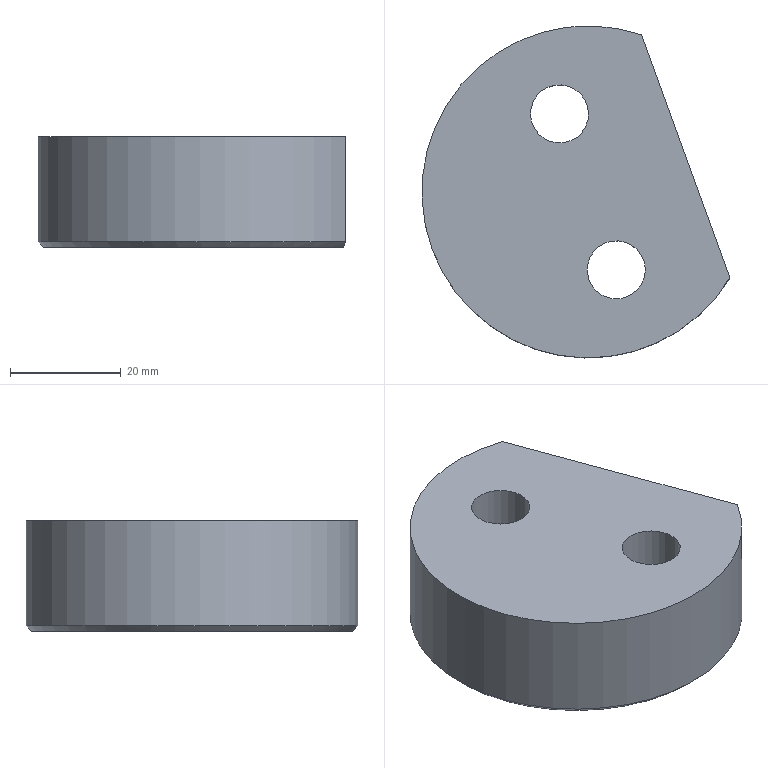Part | NX | features XD1540-60-20 2 | 1 solid | 13 faces | box 55.658 x 60 x 20 mm | volume 41796 mm3 | plane 5 | cylinder 5 | torus 2 | cone 1 | commonest cylinder face diameters 10.5 x2 17.5 x2 60 x1
STEP:
#1=CARTESIAN_POINT('',(385.107,-197.818,-380.));
#2=VERTEX_POINT('',#1);
#3=CARTESIAN_POINT('',(400.214,-239.326,-380.));
#4=VERTEX_POINT('',#3);
#5=CARTESIAN_POINT('',(392.66,-218.572,-380.));
#6=DIRECTION('',(0.342,-0.9397,0.));
#7=VECTOR('',#6,1000.);
#8=LINE('',#5,#7);
#9=EDGE_CURVE('',#2,#4,#8,.T.);
#10=ORIENTED_EDGE('',*,*,#9,.T.);
#11=CARTESIAN_POINT('',(375.,-225.,-380.));
#12=DIRECTION('',(0.,0.,1.));
#13=DIRECTION('',(0.9063,-0.4226,0.));
#14=AXIS2_PLACEMENT_3D('',#11,#12,#13);
#15=CIRCLE('',#14,29.);
#16=EDGE_CURVE('',#2,#4,#15,.T.);
#17=ORIENTED_EDGE('',*,*,#16,.F.);
#18=EDGE_LOOP('',(#10,#17));
#19=FACE_BOUND('',#18,.T.);
#20=CARTESIAN_POINT('',(390.779,-244.061,-380.));
#21=VERTEX_POINT('',#20);
#22=CARTESIAN_POINT('',(380.13,-239.095,-380.));
#23=DIRECTION('',(0.,0.,-1.));
#24=DIRECTION('',(0.9063,-0.4226,0.));
#25=AXIS2_PLACEMENT_3D('',#22,#23,#24);
#26=CIRCLE('',#25,11.75);
#27=EDGE_CURVE('',#21,#21,#26,.T.);
#28=ORIENTED_EDGE('',*,*,#27,.F.);
#29=EDGE_LOOP('',(#28));
#30=FACE_BOUND('',#29,.T.);
#31=CARTESIAN_POINT('',(380.519,-215.87,-380.));
#32=VERTEX_POINT('',#31);
#33=CARTESIAN_POINT('',(369.87,-210.905,-380.));
#34=DIRECTION('',(0.,0.,-1.));
#35=DIRECTION('',(0.9063,-0.4226,0.));
#36=AXIS2_PLACEMENT_3D('',#33,#34,#35);
#37=CIRCLE('',#36,11.75);
#38=EDGE_CURVE('',#32,#32,#37,.T.);
#39=ORIENTED_EDGE('',*,*,#38,.F.);
#40=EDGE_LOOP('',(#39));
#41=FACE_BOUND('',#40,.T.);
#42=CARTESIAN_POINT('',(375.,-225.,-380.));
#43=DIRECTION('',(0.,0.,-1.));
#44=DIRECTION('',(-0.9063,0.4226,0.));
#45=AXIS2_PLACEMENT_3D('',#42,#43,#44);
#46=PLANE('',#45);
#47=ADVANCED_FACE('',(#19,#30,#41),#46,.T.);
#48=CARTESIAN_POINT('',(400.658,-240.545,-360.));
#49=VERTEX_POINT('',#48);
#50=CARTESIAN_POINT('',(384.663,-196.599,-360.));
#51=VERTEX_POINT('',#50);
#52=CARTESIAN_POINT('',(392.66,-218.572,-360.));
#53=DIRECTION('',(-0.342,0.9397,0.));
#54=VECTOR('',#53,1000.);
#55=LINE('',#52,#54);
#56=EDGE_CURVE('',#49,#51,#55,.T.);
#57=ORIENTED_EDGE('',*,*,#56,.T.);
#58=CARTESIAN_POINT('',(375.,-225.,-360.));
#59=DIRECTION('',(0.,0.,1.));
#60=DIRECTION('',(0.9063,-0.4226,0.));
#61=AXIS2_PLACEMENT_3D('',#58,#59,#60);
#62=CIRCLE('',#61,30.);
#63=EDGE_CURVE('',#51,#49,#62,.T.);
#64=ORIENTED_EDGE('',*,*,#63,.T.);
#65=EDGE_LOOP('',(#57,#64));
#66=FACE_BOUND('',#65,.T.);
#67=CARTESIAN_POINT('',(375.372,-236.877,-360.));
#68=VERTEX_POINT('',#67);
#69=CARTESIAN_POINT('',(380.13,-239.095,-360.));
#70=DIRECTION('',(0.,0.,-1.));
#71=DIRECTION('',(-0.9063,0.4226,0.));
#72=AXIS2_PLACEMENT_3D('',#69,#70,#71);
#73=CIRCLE('',#72,5.25);
#74=EDGE_CURVE('',#68,#68,#73,.T.);
#75=ORIENTED_EDGE('',*,*,#74,.T.);
#76=EDGE_LOOP('',(#75));
#77=FACE_BOUND('',#76,.T.);
#78=CARTESIAN_POINT('',(365.112,-208.686,-360.));
#79=VERTEX_POINT('',#78);
#80=CARTESIAN_POINT('',(369.87,-210.905,-360.));
#81=DIRECTION('',(0.,0.,-1.));
#82=DIRECTION('',(-0.9063,0.4226,0.));
#83=AXIS2_PLACEMENT_3D('',#80,#81,#82);
#84=CIRCLE('',#83,5.25);
#85=EDGE_CURVE('',#79,#79,#84,.T.);
#86=ORIENTED_EDGE('',*,*,#85,.T.);
#87=EDGE_LOOP('',(#86));
#88=FACE_BOUND('',#87,.T.);
#89=CARTESIAN_POINT('',(375.,-225.,-360.));
#90=DIRECTION('',(0.,0.,1.));
#91=DIRECTION('',(0.9063,-0.4226,0.));
#92=AXIS2_PLACEMENT_3D('',#89,#90,#91);
#93=PLANE('',#92);
#94=ADVANCED_FACE('',(#66,#77,#88),#93,.T.);
#95=CARTESIAN_POINT('',(400.658,-240.545,-379.));
#96=VERTEX_POINT('',#95);
#97=CARTESIAN_POINT('',(400.658,-240.545,-360.));
#98=DIRECTION('',(0.,0.,1.));
#99=VECTOR('',#98,1000.);
#100=LINE('',#97,#99);
#101=EDGE_CURVE('',#96,#49,#100,.T.);
#102=ORIENTED_EDGE('',*,*,#101,.T.);
#103=ORIENTED_EDGE('',*,*,#63,.F.);
#104=CARTESIAN_POINT('',(384.663,-196.599,-379.));
#105=VERTEX_POINT('',#104);
#106=CARTESIAN_POINT('',(384.663,-196.599,-360.));
#107=DIRECTION('',(0.,0.,-1.));
#108=VECTOR('',#107,1000.);
#109=LINE('',#106,#108);
#110=EDGE_CURVE('',#51,#105,#109,.T.);
#111=ORIENTED_EDGE('',*,*,#110,.T.);
#112=CARTESIAN_POINT('',(375.,-225.,-379.));
#113=DIRECTION('',(0.,0.,-1.));
#114=DIRECTION('',(0.9063,-0.4226,0.));
#115=AXIS2_PLACEMENT_3D('',#112,#113,#114);
#116=CIRCLE('',#115,30.);
#117=EDGE_CURVE('',#96,#105,#116,.T.);
#118=ORIENTED_EDGE('',*,*,#117,.F.);
#119=EDGE_LOOP('',(#102,#103,#111,#118));
#120=FACE_BOUND('',#119,.T.);
#121=CARTESIAN_POINT('',(375.,-225.,-360.));
#122=DIRECTION('',(0.,0.,-1.));
#123=DIRECTION('',(-0.9063,0.4226,0.));
#124=AXIS2_PLACEMENT_3D('',#121,#122,#123);
#125=CYLINDRICAL_SURFACE('',#124,30.);
#126=ADVANCED_FACE('',(#120),#125,.T.);
#127=CARTESIAN_POINT('',(365.112,-208.686,-368.));
#128=VERTEX_POINT('',#127);
#129=CARTESIAN_POINT('',(369.87,-210.905,-368.));
#130=DIRECTION('',(0.,0.,-1.));
#131=DIRECTION('',(-0.9063,0.4226,0.));
#132=AXIS2_PLACEMENT_3D('',#129,#130,#131);
#133=CIRCLE('',#132,5.25);
#134=EDGE_CURVE('',#128,#128,#133,.T.);
#135=ORIENTED_EDGE('',*,*,#134,.F.);
#136=EDGE_LOOP('',(#135));
#137=FACE_BOUND('',#136,.T.);
#138=CARTESIAN_POINT('',(377.8,-214.603,-368.));
#139=VERTEX_POINT('',#138);
#140=CARTESIAN_POINT('',(369.87,-210.905,-368.));
#141=DIRECTION('',(0.,0.,1.));
#142=DIRECTION('',(0.9063,-0.4226,0.));
#143=AXIS2_PLACEMENT_3D('',#140,#141,#142);
#144=CIRCLE('',#143,8.75);
#145=EDGE_CURVE('',#139,#139,#144,.T.);
#146=ORIENTED_EDGE('',*,*,#145,.F.);
#147=EDGE_LOOP('',(#146));
#148=FACE_BOUND('',#147,.T.);
#149=CARTESIAN_POINT('',(369.87,-210.905,-368.));
#150=DIRECTION('',(0.,0.,1.));
#151=DIRECTION('',(0.9063,-0.4226,0.));
#152=AXIS2_PLACEMENT_3D('',#149,#150,#151);
#153=PLANE('',#152);
#154=ADVANCED_FACE('',(#137,#148),#153,.F.);
#155=CARTESIAN_POINT('',(377.8,-214.603,-377.));
#156=VERTEX_POINT('',#155);
#157=CARTESIAN_POINT('',(369.87,-210.905,-377.));
#158=DIRECTION('',(0.,0.,1.));
#159=DIRECTION('',(0.9063,-0.4226,0.));
#160=AXIS2_PLACEMENT_3D('',#157,#158,#159);
#161=CIRCLE('',#160,8.75);
#162=EDGE_CURVE('',#156,#156,#161,.T.);
#163=ORIENTED_EDGE('',*,*,#162,.F.);
#164=EDGE_LOOP('',(#163));
#165=FACE_BOUND('',#164,.T.);
#166=ORIENTED_EDGE('',*,*,#145,.T.);
#167=EDGE_LOOP('',(#166));
#168=FACE_BOUND('',#167,.T.);
#169=CARTESIAN_POINT('',(369.87,-210.905,-368.));
#170=DIRECTION('',(0.,0.,-1.));
#171=DIRECTION('',(-0.9063,0.4226,0.));
#172=AXIS2_PLACEMENT_3D('',#169,#170,#171);
#173=CYLINDRICAL_SURFACE('',#172,8.75);
#174=ADVANCED_FACE('',(#165,#168),#173,.F.);
#175=CARTESIAN_POINT('',(375.372,-236.877,-368.));
#176=VERTEX_POINT('',#175);
#177=CARTESIAN_POINT('',(380.13,-239.095,-368.));
#178=DIRECTION('',(0.,0.,-1.));
#179=DIRECTION('',(-0.9063,0.4226,0.));
#180=AXIS2_PLACEMENT_3D('',#177,#178,#179);
#181=CIRCLE('',#180,5.25);
#182=EDGE_CURVE('',#176,#176,#181,.T.);
#183=ORIENTED_EDGE('',*,*,#182,.F.);
#184=EDGE_LOOP('',(#183));
#185=FACE_BOUND('',#184,.T.);
#186=CARTESIAN_POINT('',(388.06,-242.793,-368.));
#187=VERTEX_POINT('',#186);
#188=CARTESIAN_POINT('',(380.13,-239.095,-368.));
#189=DIRECTION('',(0.,0.,1.));
#190=DIRECTION('',(0.9063,-0.4226,0.));
#191=AXIS2_PLACEMENT_3D('',#188,#189,#190);
#192=CIRCLE('',#191,8.75);
#193=EDGE_CURVE('',#187,#187,#192,.T.);
#194=ORIENTED_EDGE('',*,*,#193,.F.);
#195=EDGE_LOOP('',(#194));
#196=FACE_BOUND('',#195,.T.);
#197=CARTESIAN_POINT('',(380.13,-239.095,-368.));
#198=DIRECTION('',(0.,0.,1.));
#199=DIRECTION('',(0.9063,-0.4226,0.));
#200=AXIS2_PLACEMENT_3D('',#197,#198,#199);
#201=PLANE('',#200);
#202=ADVANCED_FACE('',(#185,#196),#201,.F.);
#203=CARTESIAN_POINT('',(388.06,-242.793,-377.));
#204=VERTEX_POINT('',#203);
#205=CARTESIAN_POINT('',(380.13,-239.095,-377.));
#206=DIRECTION('',(0.,0.,1.));
#207=DIRECTION('',(0.9063,-0.4226,0.));
#208=AXIS2_PLACEMENT_3D('',#205,#206,#207);
#209=CIRCLE('',#208,8.75);
#210=EDGE_CURVE('',#204,#204,#209,.T.);
#211=ORIENTED_EDGE('',*,*,#210,.F.);
#212=EDGE_LOOP('',(#211));
#213=FACE_BOUND('',#212,.T.);
#214=ORIENTED_EDGE('',*,*,#193,.T.);
#215=EDGE_LOOP('',(#214));
#216=FACE_BOUND('',#215,.T.);
#217=CARTESIAN_POINT('',(380.13,-239.095,-368.));
#218=DIRECTION('',(0.,0.,-1.));
#219=DIRECTION('',(-0.9063,0.4226,0.));
#220=AXIS2_PLACEMENT_3D('',#217,#218,#219);
#221=CYLINDRICAL_SURFACE('',#220,8.75);
#222=ADVANCED_FACE('',(#213,#216),#221,.F.);
#223=ORIENTED_EDGE('',*,*,#85,.F.);
#224=EDGE_LOOP('',(#223));
#225=FACE_BOUND('',#224,.T.);
#226=ORIENTED_EDGE('',*,*,#134,.T.);
#227=EDGE_LOOP('',(#226));
#228=FACE_BOUND('',#227,.T.);
#229=CARTESIAN_POINT('',(369.87,-210.905,-359.));
#230=DIRECTION('',(0.,0.,-1.));
#231=DIRECTION('',(-0.9063,0.4226,0.));
#232=AXIS2_PLACEMENT_3D('',#229,#230,#231);
#233=CYLINDRICAL_SURFACE('',#232,5.25);
#234=ADVANCED_FACE('',(#225,#228),#233,.F.);
#235=ORIENTED_EDGE('',*,*,#74,.F.);
#236=EDGE_LOOP('',(#235));
#237=FACE_BOUND('',#236,.T.);
#238=ORIENTED_EDGE('',*,*,#182,.T.);
#239=EDGE_LOOP('',(#238));
#240=FACE_BOUND('',#239,.T.);
#241=CARTESIAN_POINT('',(380.13,-239.095,-359.));
#242=DIRECTION('',(0.,0.,-1.));
#243=DIRECTION('',(-0.9063,0.4226,0.));
#244=AXIS2_PLACEMENT_3D('',#241,#242,#243);
#245=CYLINDRICAL_SURFACE('',#244,5.25);
#246=ADVANCED_FACE('',(#237,#240),#245,.F.);
#247=ORIENTED_EDGE('',*,*,#38,.T.);
#248=EDGE_LOOP('',(#247));
#249=FACE_BOUND('',#248,.T.);
#250=ORIENTED_EDGE('',*,*,#162,.T.);
#251=EDGE_LOOP('',(#250));
#252=FACE_BOUND('',#251,.T.);
#253=CARTESIAN_POINT('',(369.87,-210.905,-377.));
#254=DIRECTION('',(0.,0.,-1.));
#255=DIRECTION('',(-0.9063,0.4226,0.));
#256=AXIS2_PLACEMENT_3D('',#253,#254,#255);
#257=TOROIDAL_SURFACE('',#256,11.75,3.);
#258=ADVANCED_FACE('',(#249,#252),#257,.T.);
#259=ORIENTED_EDGE('',*,*,#27,.T.);
#260=EDGE_LOOP('',(#259));
#261=FACE_BOUND('',#260,.T.);
#262=ORIENTED_EDGE('',*,*,#210,.T.);
#263=EDGE_LOOP('',(#262));
#264=FACE_BOUND('',#263,.T.);
#265=CARTESIAN_POINT('',(380.13,-239.095,-377.));
#266=DIRECTION('',(0.,0.,-1.));
#267=DIRECTION('',(-0.9063,0.4226,0.));
#268=AXIS2_PLACEMENT_3D('',#265,#266,#267);
#269=TOROIDAL_SURFACE('',#268,11.75,3.);
#270=ADVANCED_FACE('',(#261,#264),#269,.T.);
#271=CARTESIAN_POINT('',(384.663,-196.599,-379.));
#272=CARTESIAN_POINT('',(384.81,-197.003,-379.336));
#273=CARTESIAN_POINT('',(384.958,-197.41,-379.669));
#274=CARTESIAN_POINT('',(385.107,-197.818,-380.));
#275=B_SPLINE_CURVE_WITH_KNOTS('',3,(#271,#272,#273,#274),.UNSPECIFIED.,.F.,.F.,(4,4),(0.,1.),.PIECEWISE_BEZIER_KNOTS.);
#276=EDGE_CURVE('',#105,#2,#275,.T.);
#277=ORIENTED_EDGE('',*,*,#276,.T.);
#278=ORIENTED_EDGE('',*,*,#16,.T.);
#279=CARTESIAN_POINT('',(400.214,-239.326,-380.));
#280=CARTESIAN_POINT('',(400.363,-239.734,-379.669));
#281=CARTESIAN_POINT('',(400.511,-240.141,-379.336));
#282=CARTESIAN_POINT('',(400.658,-240.545,-379.));
#283=B_SPLINE_CURVE_WITH_KNOTS('',3,(#279,#280,#281,#282),.UNSPECIFIED.,.F.,.F.,(4,4),(0.,1.),.PIECEWISE_BEZIER_KNOTS.);
#284=EDGE_CURVE('',#4,#96,#283,.T.);
#285=ORIENTED_EDGE('',*,*,#284,.T.);
#286=ORIENTED_EDGE('',*,*,#117,.T.);
#287=EDGE_LOOP('',(#277,#278,#285,#286));
#288=FACE_BOUND('',#287,.T.);
#289=CARTESIAN_POINT('',(375.,-225.,-379.));
#290=DIRECTION('',(0.,0.,1.));
#291=DIRECTION('',(0.9063,-0.4226,0.));
#292=AXIS2_PLACEMENT_3D('',#289,#290,#291);
#293=CONICAL_SURFACE('',#292,30.,0.7854);
#294=ADVANCED_FACE('',(#288),#293,.T.);
#295=ORIENTED_EDGE('',*,*,#110,.F.);
#296=ORIENTED_EDGE('',*,*,#56,.F.);
#297=ORIENTED_EDGE('',*,*,#101,.F.);
#298=ORIENTED_EDGE('',*,*,#284,.F.);
#299=ORIENTED_EDGE('',*,*,#9,.F.);
#300=ORIENTED_EDGE('',*,*,#276,.F.);
#301=EDGE_LOOP('',(#295,#296,#297,#298,#299,#300));
#302=FACE_BOUND('',#301,.T.);
#303=CARTESIAN_POINT('',(404.919,-252.251,-580.));
#304=DIRECTION('',(-0.9397,-0.342,0.));
#305=DIRECTION('',(0.342,-0.9397,0.));
#306=AXIS2_PLACEMENT_3D('',#303,#304,#305);
#307=PLANE('',#306);
#308=ADVANCED_FACE('',(#302),#307,.F.);
#309=CLOSED_SHELL('',(#47,#94,#126,#154,#174,#202,#222,#234,#246,#258,#270,#294,#308));
#310=MANIFOLD_SOLID_BREP('',#309);
#311=(LENGTH_UNIT()NAMED_UNIT(*)SI_UNIT(.MILLI.,.METRE.));
#312=UNCERTAINTY_MEASURE_WITH_UNIT(LENGTH_MEASURE(0.00001),#311,'','');
#313=(NAMED_UNIT(*)PLANE_ANGLE_UNIT()SI_UNIT($,.RADIAN.));
#314=(NAMED_UNIT(*)SI_UNIT($,.STERADIAN.)SOLID_ANGLE_UNIT());
#315=(GEOMETRIC_REPRESENTATION_CONTEXT(3)GLOBAL_UNCERTAINTY_ASSIGNED_CONTEXT((#312))GLOBAL_UNIT_ASSIGNED_CONTEXT((#311,#313,#314))REPRESENTATION_CONTEXT('',''));
#316=ADVANCED_BREP_SHAPE_REPRESENTATION('',(#310),#315);